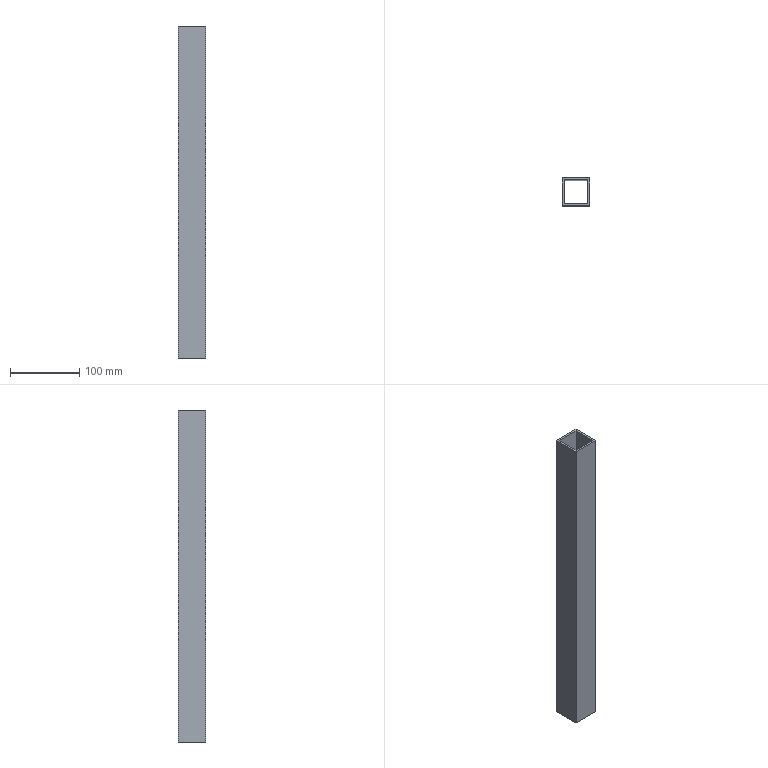Part | STEP file | BCC3 H18_2 | 1 solid | 10 faces | box 40 x 40 x 480 mm | volume 213120 mm3 | plane 10
STEP:
#1=CARTESIAN_POINT('',(0.,0.,0.));
#2=DIRECTION('',(0.,0.,1.));
#3=DIRECTION('',(1.,0.,0.));
#4=AXIS2_PLACEMENT_3D('',#1,#2,#3);
#5=CARTESIAN_POINT('',(-20.,20.,240.));
#6=VERTEX_POINT('',#5);
#7=CARTESIAN_POINT('',(-20.,-20.,240.));
#8=VERTEX_POINT('',#7);
#9=CARTESIAN_POINT('',(-20.,20.,240.));
#10=DIRECTION('',(0.,-1.,0.));
#11=VECTOR('',#10,1.);
#12=LINE('',#9,#11);
#13=CARTESIAN_POINT('',(0.,0.,240.));
#14=DIRECTION('',(0.,0.,1.));
#15=DIRECTION('',(1.,0.,0.));
#16=AXIS2_PLACEMENT_3D('',#13,#14,#15);
#17=PLANE('',#16);
#18=CARTESIAN_POINT('',(-20.,20.));
#19=DIRECTION('',(0.,-1.));
#20=VECTOR('',#19,1.);
#21=LINE('',#18,#20);
#22=(GEOMETRIC_REPRESENTATION_CONTEXT(2)PARAMETRIC_REPRESENTATION_CONTEXT()REPRESENTATION_CONTEXT('',''));
#23=DEFINITIONAL_REPRESENTATION('',(#21),#22);
#24=PCURVE('',#17,#23);
#25=CARTESIAN_POINT('',(-20.,20.,240.));
#26=DIRECTION('',(1.,0.,0.));
#27=DIRECTION('',(0.,1.,0.));
#28=AXIS2_PLACEMENT_3D('',#25,#26,#27);
#29=PLANE('',#28);
#30=CARTESIAN_POINT('',(0.,0.));
#31=DIRECTION('',(-1.,0.));
#32=VECTOR('',#31,1.);
#33=LINE('',#30,#32);
#34=(GEOMETRIC_REPRESENTATION_CONTEXT(2)PARAMETRIC_REPRESENTATION_CONTEXT()REPRESENTATION_CONTEXT('',''));
#35=DEFINITIONAL_REPRESENTATION('',(#33),#34);
#36=PCURVE('',#29,#35);
#37=SURFACE_CURVE('',#12,(#24,#36),.PCURVE_S1.);
#38=EDGE_CURVE('',#6,#8,#37,.T.);
#39=ORIENTED_EDGE('',*,*,#38,.T.);
#40=CARTESIAN_POINT('',(20.,-20.,240.));
#41=VERTEX_POINT('',#40);
#42=CARTESIAN_POINT('',(-20.,-20.,240.));
#43=DIRECTION('',(1.,0.,0.));
#44=VECTOR('',#43,1.);
#45=LINE('',#42,#44);
#46=CARTESIAN_POINT('',(-20.,-20.));
#47=DIRECTION('',(1.,0.));
#48=VECTOR('',#47,1.);
#49=LINE('',#46,#48);
#50=(GEOMETRIC_REPRESENTATION_CONTEXT(2)PARAMETRIC_REPRESENTATION_CONTEXT()REPRESENTATION_CONTEXT('',''));
#51=DEFINITIONAL_REPRESENTATION('',(#49),#50);
#52=PCURVE('',#17,#51);
#53=CARTESIAN_POINT('',(-20.,-20.,240.));
#54=DIRECTION('',(0.,1.,0.));
#55=DIRECTION('',(0.,0.,1.));
#56=AXIS2_PLACEMENT_3D('',#53,#54,#55);
#57=PLANE('',#56);
#58=CARTESIAN_POINT('',(0.,0.));
#59=DIRECTION('',(0.,1.));
#60=VECTOR('',#59,1.);
#61=LINE('',#58,#60);
#62=(GEOMETRIC_REPRESENTATION_CONTEXT(2)PARAMETRIC_REPRESENTATION_CONTEXT()REPRESENTATION_CONTEXT('',''));
#63=DEFINITIONAL_REPRESENTATION('',(#61),#62);
#64=PCURVE('',#57,#63);
#65=SURFACE_CURVE('',#45,(#52,#64),.PCURVE_S1.);
#66=EDGE_CURVE('',#8,#41,#65,.T.);
#67=ORIENTED_EDGE('',*,*,#66,.T.);
#68=CARTESIAN_POINT('',(20.,20.,240.));
#69=VERTEX_POINT('',#68);
#70=CARTESIAN_POINT('',(20.,20.,240.));
#71=DIRECTION('',(0.,1.,0.));
#72=VECTOR('',#71,1.);
#73=LINE('',#70,#72);
#74=CARTESIAN_POINT('',(20.,20.));
#75=DIRECTION('',(0.,1.));
#76=VECTOR('',#75,1.);
#77=LINE('',#74,#76);
#78=(GEOMETRIC_REPRESENTATION_CONTEXT(2)PARAMETRIC_REPRESENTATION_CONTEXT()REPRESENTATION_CONTEXT('',''));
#79=DEFINITIONAL_REPRESENTATION('',(#77),#78);
#80=PCURVE('',#17,#79);
#81=CARTESIAN_POINT('',(20.,20.,240.));
#82=DIRECTION('',(-1.,0.,0.));
#83=DIRECTION('',(0.,-1.,0.));
#84=AXIS2_PLACEMENT_3D('',#81,#82,#83);
#85=PLANE('',#84);
#86=CARTESIAN_POINT('',(0.,0.));
#87=DIRECTION('',(-1.,0.));
#88=VECTOR('',#87,1.);
#89=LINE('',#86,#88);
#90=(GEOMETRIC_REPRESENTATION_CONTEXT(2)PARAMETRIC_REPRESENTATION_CONTEXT()REPRESENTATION_CONTEXT('',''));
#91=DEFINITIONAL_REPRESENTATION('',(#89),#90);
#92=PCURVE('',#85,#91);
#93=SURFACE_CURVE('',#73,(#80,#92),.PCURVE_S1.);
#94=EDGE_CURVE('',#41,#69,#93,.T.);
#95=ORIENTED_EDGE('',*,*,#94,.T.);
#96=CARTESIAN_POINT('',(-20.,20.,240.));
#97=DIRECTION('',(-1.,0.,0.));
#98=VECTOR('',#97,1.);
#99=LINE('',#96,#98);
#100=CARTESIAN_POINT('',(-20.,20.));
#101=DIRECTION('',(-1.,0.));
#102=VECTOR('',#101,1.);
#103=LINE('',#100,#102);
#104=(GEOMETRIC_REPRESENTATION_CONTEXT(2)PARAMETRIC_REPRESENTATION_CONTEXT()REPRESENTATION_CONTEXT('',''));
#105=DEFINITIONAL_REPRESENTATION('',(#103),#104);
#106=PCURVE('',#17,#105);
#107=CARTESIAN_POINT('',(-20.,20.,240.));
#108=DIRECTION('',(0.,-1.,0.));
#109=DIRECTION('',(0.,0.,-1.));
#110=AXIS2_PLACEMENT_3D('',#107,#108,#109);
#111=PLANE('',#110);
#112=CARTESIAN_POINT('',(0.,0.));
#113=DIRECTION('',(0.,-1.));
#114=VECTOR('',#113,1.);
#115=LINE('',#112,#114);
#116=(GEOMETRIC_REPRESENTATION_CONTEXT(2)PARAMETRIC_REPRESENTATION_CONTEXT()REPRESENTATION_CONTEXT('',''));
#117=DEFINITIONAL_REPRESENTATION('',(#115),#116);
#118=PCURVE('',#111,#117);
#119=SURFACE_CURVE('',#99,(#106,#118),.PCURVE_S1.);
#120=EDGE_CURVE('',#69,#6,#119,.T.);
#121=ORIENTED_EDGE('',*,*,#120,.T.);
#122=EDGE_LOOP('',(#39,#67,#95,#121));
#123=FACE_BOUND('',#122,.T.);
#124=CARTESIAN_POINT('',(-17.,-17.,240.));
#125=VERTEX_POINT('',#124);
#126=CARTESIAN_POINT('',(17.,-17.,240.));
#127=VERTEX_POINT('',#126);
#128=CARTESIAN_POINT('',(-17.,-17.,240.));
#129=DIRECTION('',(1.,0.,0.));
#130=VECTOR('',#129,1.);
#131=LINE('',#128,#130);
#132=CARTESIAN_POINT('',(-17.,-17.));
#133=DIRECTION('',(1.,0.));
#134=VECTOR('',#133,1.);
#135=LINE('',#132,#134);
#136=(GEOMETRIC_REPRESENTATION_CONTEXT(2)PARAMETRIC_REPRESENTATION_CONTEXT()REPRESENTATION_CONTEXT('',''));
#137=DEFINITIONAL_REPRESENTATION('',(#135),#136);
#138=PCURVE('',#17,#137);
#139=CARTESIAN_POINT('',(-17.,-17.,240.));
#140=DIRECTION('',(0.,1.,0.));
#141=DIRECTION('',(-1.,0.,0.));
#142=AXIS2_PLACEMENT_3D('',#139,#140,#141);
#143=PLANE('',#142);
#144=CARTESIAN_POINT('',(0.,0.));
#145=DIRECTION('',(-1.,0.));
#146=VECTOR('',#145,1.);
#147=LINE('',#144,#146);
#148=(GEOMETRIC_REPRESENTATION_CONTEXT(2)PARAMETRIC_REPRESENTATION_CONTEXT()REPRESENTATION_CONTEXT('',''));
#149=DEFINITIONAL_REPRESENTATION('',(#147),#148);
#150=PCURVE('',#143,#149);
#151=SURFACE_CURVE('',#131,(#138,#150),.PCURVE_S1.);
#152=EDGE_CURVE('',#125,#127,#151,.T.);
#153=ORIENTED_EDGE('',*,*,#152,.F.);
#154=CARTESIAN_POINT('',(-17.,17.,240.));
#155=VERTEX_POINT('',#154);
#156=CARTESIAN_POINT('',(-17.,17.,240.));
#157=DIRECTION('',(0.,-1.,0.));
#158=VECTOR('',#157,1.);
#159=LINE('',#156,#158);
#160=CARTESIAN_POINT('',(-17.,17.));
#161=DIRECTION('',(0.,-1.));
#162=VECTOR('',#161,1.);
#163=LINE('',#160,#162);
#164=(GEOMETRIC_REPRESENTATION_CONTEXT(2)PARAMETRIC_REPRESENTATION_CONTEXT()REPRESENTATION_CONTEXT('',''));
#165=DEFINITIONAL_REPRESENTATION('',(#163),#164);
#166=PCURVE('',#17,#165);
#167=CARTESIAN_POINT('',(-17.,17.,240.));
#168=DIRECTION('',(1.,0.,0.));
#169=DIRECTION('',(0.,1.,0.));
#170=AXIS2_PLACEMENT_3D('',#167,#168,#169);
#171=PLANE('',#170);
#172=CARTESIAN_POINT('',(0.,0.));
#173=DIRECTION('',(-1.,0.));
#174=VECTOR('',#173,1.);
#175=LINE('',#172,#174);
#176=(GEOMETRIC_REPRESENTATION_CONTEXT(2)PARAMETRIC_REPRESENTATION_CONTEXT()REPRESENTATION_CONTEXT('',''));
#177=DEFINITIONAL_REPRESENTATION('',(#175),#176);
#178=PCURVE('',#171,#177);
#179=SURFACE_CURVE('',#159,(#166,#178),.PCURVE_S1.);
#180=EDGE_CURVE('',#155,#125,#179,.T.);
#181=ORIENTED_EDGE('',*,*,#180,.F.);
#182=CARTESIAN_POINT('',(17.,17.,240.));
#183=VERTEX_POINT('',#182);
#184=CARTESIAN_POINT('',(-17.,17.,240.));
#185=DIRECTION('',(-1.,0.,0.));
#186=VECTOR('',#185,1.);
#187=LINE('',#184,#186);
#188=CARTESIAN_POINT('',(-17.,17.));
#189=DIRECTION('',(-1.,0.));
#190=VECTOR('',#189,1.);
#191=LINE('',#188,#190);
#192=(GEOMETRIC_REPRESENTATION_CONTEXT(2)PARAMETRIC_REPRESENTATION_CONTEXT()REPRESENTATION_CONTEXT('',''));
#193=DEFINITIONAL_REPRESENTATION('',(#191),#192);
#194=PCURVE('',#17,#193);
#195=CARTESIAN_POINT('',(-17.,17.,240.));
#196=DIRECTION('',(0.,-1.,0.));
#197=DIRECTION('',(0.,0.,-1.));
#198=AXIS2_PLACEMENT_3D('',#195,#196,#197);
#199=PLANE('',#198);
#200=CARTESIAN_POINT('',(0.,0.));
#201=DIRECTION('',(0.,-1.));
#202=VECTOR('',#201,1.);
#203=LINE('',#200,#202);
#204=(GEOMETRIC_REPRESENTATION_CONTEXT(2)PARAMETRIC_REPRESENTATION_CONTEXT()REPRESENTATION_CONTEXT('',''));
#205=DEFINITIONAL_REPRESENTATION('',(#203),#204);
#206=PCURVE('',#199,#205);
#207=SURFACE_CURVE('',#187,(#194,#206),.PCURVE_S1.);
#208=EDGE_CURVE('',#183,#155,#207,.T.);
#209=ORIENTED_EDGE('',*,*,#208,.F.);
#210=CARTESIAN_POINT('',(17.,17.,240.));
#211=DIRECTION('',(0.,1.,0.));
#212=VECTOR('',#211,1.);
#213=LINE('',#210,#212);
#214=CARTESIAN_POINT('',(17.,17.));
#215=DIRECTION('',(0.,1.));
#216=VECTOR('',#215,1.);
#217=LINE('',#214,#216);
#218=(GEOMETRIC_REPRESENTATION_CONTEXT(2)PARAMETRIC_REPRESENTATION_CONTEXT()REPRESENTATION_CONTEXT('',''));
#219=DEFINITIONAL_REPRESENTATION('',(#217),#218);
#220=PCURVE('',#17,#219);
#221=CARTESIAN_POINT('',(17.,17.,240.));
#222=DIRECTION('',(-1.,0.,0.));
#223=DIRECTION('',(0.,-1.,0.));
#224=AXIS2_PLACEMENT_3D('',#221,#222,#223);
#225=PLANE('',#224);
#226=CARTESIAN_POINT('',(0.,0.));
#227=DIRECTION('',(-1.,0.));
#228=VECTOR('',#227,1.);
#229=LINE('',#226,#228);
#230=(GEOMETRIC_REPRESENTATION_CONTEXT(2)PARAMETRIC_REPRESENTATION_CONTEXT()REPRESENTATION_CONTEXT('',''));
#231=DEFINITIONAL_REPRESENTATION('',(#229),#230);
#232=PCURVE('',#225,#231);
#233=SURFACE_CURVE('',#213,(#220,#232),.PCURVE_S1.);
#234=EDGE_CURVE('',#127,#183,#233,.T.);
#235=ORIENTED_EDGE('',*,*,#234,.F.);
#236=EDGE_LOOP('',(#153,#181,#209,#235));
#237=FACE_BOUND('',#236,.T.);
#238=ADVANCED_FACE('',(#123,#237),#17,.T.);
#239=CARTESIAN_POINT('',(-20.,20.,-240.));
#240=VERTEX_POINT('',#239);
#241=CARTESIAN_POINT('',(-20.,-20.,-240.));
#242=VERTEX_POINT('',#241);
#243=CARTESIAN_POINT('',(-20.,20.,-240.));
#244=DIRECTION('',(0.,-1.,0.));
#245=VECTOR('',#244,1.);
#246=LINE('',#243,#245);
#247=CARTESIAN_POINT('',(0.,0.,-240.));
#248=DIRECTION('',(0.,0.,1.));
#249=DIRECTION('',(1.,0.,0.));
#250=AXIS2_PLACEMENT_3D('',#247,#248,#249);
#251=PLANE('',#250);
#252=CARTESIAN_POINT('',(-20.,20.));
#253=DIRECTION('',(0.,-1.));
#254=VECTOR('',#253,1.);
#255=LINE('',#252,#254);
#256=(GEOMETRIC_REPRESENTATION_CONTEXT(2)PARAMETRIC_REPRESENTATION_CONTEXT()REPRESENTATION_CONTEXT('',''));
#257=DEFINITIONAL_REPRESENTATION('',(#255),#256);
#258=PCURVE('',#251,#257);
#259=CARTESIAN_POINT('',(0.,-480.));
#260=DIRECTION('',(-1.,0.));
#261=VECTOR('',#260,1.);
#262=LINE('',#259,#261);
#263=(GEOMETRIC_REPRESENTATION_CONTEXT(2)PARAMETRIC_REPRESENTATION_CONTEXT()REPRESENTATION_CONTEXT('',''));
#264=DEFINITIONAL_REPRESENTATION('',(#262),#263);
#265=PCURVE('',#29,#264);
#266=SURFACE_CURVE('',#246,(#258,#265),.PCURVE_S1.);
#267=EDGE_CURVE('',#240,#242,#266,.T.);
#268=ORIENTED_EDGE('',*,*,#267,.F.);
#269=CARTESIAN_POINT('',(20.,20.,-240.));
#270=VERTEX_POINT('',#269);
#271=CARTESIAN_POINT('',(-20.,20.,-240.));
#272=DIRECTION('',(-1.,0.,0.));
#273=VECTOR('',#272,1.);
#274=LINE('',#271,#273);
#275=CARTESIAN_POINT('',(-20.,20.));
#276=DIRECTION('',(-1.,0.));
#277=VECTOR('',#276,1.);
#278=LINE('',#275,#277);
#279=(GEOMETRIC_REPRESENTATION_CONTEXT(2)PARAMETRIC_REPRESENTATION_CONTEXT()REPRESENTATION_CONTEXT('',''));
#280=DEFINITIONAL_REPRESENTATION('',(#278),#279);
#281=PCURVE('',#251,#280);
#282=CARTESIAN_POINT('',(480.,0.));
#283=DIRECTION('',(0.,-1.));
#284=VECTOR('',#283,1.);
#285=LINE('',#282,#284);
#286=(GEOMETRIC_REPRESENTATION_CONTEXT(2)PARAMETRIC_REPRESENTATION_CONTEXT()REPRESENTATION_CONTEXT('',''));
#287=DEFINITIONAL_REPRESENTATION('',(#285),#286);
#288=PCURVE('',#111,#287);
#289=SURFACE_CURVE('',#274,(#281,#288),.PCURVE_S1.);
#290=EDGE_CURVE('',#270,#240,#289,.T.);
#291=ORIENTED_EDGE('',*,*,#290,.F.);
#292=CARTESIAN_POINT('',(20.,-20.,-240.));
#293=VERTEX_POINT('',#292);
#294=CARTESIAN_POINT('',(20.,20.,-240.));
#295=DIRECTION('',(0.,1.,0.));
#296=VECTOR('',#295,1.);
#297=LINE('',#294,#296);
#298=CARTESIAN_POINT('',(20.,20.));
#299=DIRECTION('',(0.,1.));
#300=VECTOR('',#299,1.);
#301=LINE('',#298,#300);
#302=(GEOMETRIC_REPRESENTATION_CONTEXT(2)PARAMETRIC_REPRESENTATION_CONTEXT()REPRESENTATION_CONTEXT('',''));
#303=DEFINITIONAL_REPRESENTATION('',(#301),#302);
#304=PCURVE('',#251,#303);
#305=CARTESIAN_POINT('',(0.,-480.));
#306=DIRECTION('',(-1.,0.));
#307=VECTOR('',#306,1.);
#308=LINE('',#305,#307);
#309=(GEOMETRIC_REPRESENTATION_CONTEXT(2)PARAMETRIC_REPRESENTATION_CONTEXT()REPRESENTATION_CONTEXT('',''));
#310=DEFINITIONAL_REPRESENTATION('',(#308),#309);
#311=PCURVE('',#85,#310);
#312=SURFACE_CURVE('',#297,(#304,#311),.PCURVE_S1.);
#313=EDGE_CURVE('',#293,#270,#312,.T.);
#314=ORIENTED_EDGE('',*,*,#313,.F.);
#315=CARTESIAN_POINT('',(-20.,-20.,-240.));
#316=DIRECTION('',(1.,0.,0.));
#317=VECTOR('',#316,1.);
#318=LINE('',#315,#317);
#319=CARTESIAN_POINT('',(-20.,-20.));
#320=DIRECTION('',(1.,0.));
#321=VECTOR('',#320,1.);
#322=LINE('',#319,#321);
#323=(GEOMETRIC_REPRESENTATION_CONTEXT(2)PARAMETRIC_REPRESENTATION_CONTEXT()REPRESENTATION_CONTEXT('',''));
#324=DEFINITIONAL_REPRESENTATION('',(#322),#323);
#325=PCURVE('',#251,#324);
#326=CARTESIAN_POINT('',(-480.,0.));
#327=DIRECTION('',(0.,1.));
#328=VECTOR('',#327,1.);
#329=LINE('',#326,#328);
#330=(GEOMETRIC_REPRESENTATION_CONTEXT(2)PARAMETRIC_REPRESENTATION_CONTEXT()REPRESENTATION_CONTEXT('',''));
#331=DEFINITIONAL_REPRESENTATION('',(#329),#330);
#332=PCURVE('',#57,#331);
#333=SURFACE_CURVE('',#318,(#325,#332),.PCURVE_S1.);
#334=EDGE_CURVE('',#242,#293,#333,.T.);
#335=ORIENTED_EDGE('',*,*,#334,.F.);
#336=EDGE_LOOP('',(#268,#291,#314,#335));
#337=FACE_BOUND('',#336,.T.);
#338=CARTESIAN_POINT('',(-17.,17.,-240.));
#339=VERTEX_POINT('',#338);
#340=CARTESIAN_POINT('',(-17.,-17.,-240.));
#341=VERTEX_POINT('',#340);
#342=CARTESIAN_POINT('',(-17.,17.,-240.));
#343=DIRECTION('',(0.,-1.,0.));
#344=VECTOR('',#343,1.);
#345=LINE('',#342,#344);
#346=CARTESIAN_POINT('',(-17.,17.));
#347=DIRECTION('',(0.,-1.));
#348=VECTOR('',#347,1.);
#349=LINE('',#346,#348);
#350=(GEOMETRIC_REPRESENTATION_CONTEXT(2)PARAMETRIC_REPRESENTATION_CONTEXT()REPRESENTATION_CONTEXT('',''));
#351=DEFINITIONAL_REPRESENTATION('',(#349),#350);
#352=PCURVE('',#251,#351);
#353=CARTESIAN_POINT('',(0.,-480.));
#354=DIRECTION('',(-1.,0.));
#355=VECTOR('',#354,1.);
#356=LINE('',#353,#355);
#357=(GEOMETRIC_REPRESENTATION_CONTEXT(2)PARAMETRIC_REPRESENTATION_CONTEXT()REPRESENTATION_CONTEXT('',''));
#358=DEFINITIONAL_REPRESENTATION('',(#356),#357);
#359=PCURVE('',#171,#358);
#360=SURFACE_CURVE('',#345,(#352,#359),.PCURVE_S1.);
#361=EDGE_CURVE('',#339,#341,#360,.T.);
#362=ORIENTED_EDGE('',*,*,#361,.T.);
#363=CARTESIAN_POINT('',(17.,-17.,-240.));
#364=VERTEX_POINT('',#363);
#365=CARTESIAN_POINT('',(-17.,-17.,-240.));
#366=DIRECTION('',(1.,0.,0.));
#367=VECTOR('',#366,1.);
#368=LINE('',#365,#367);
#369=CARTESIAN_POINT('',(-17.,-17.));
#370=DIRECTION('',(1.,0.));
#371=VECTOR('',#370,1.);
#372=LINE('',#369,#371);
#373=(GEOMETRIC_REPRESENTATION_CONTEXT(2)PARAMETRIC_REPRESENTATION_CONTEXT()REPRESENTATION_CONTEXT('',''));
#374=DEFINITIONAL_REPRESENTATION('',(#372),#373);
#375=PCURVE('',#251,#374);
#376=CARTESIAN_POINT('',(0.,-480.));
#377=DIRECTION('',(-1.,0.));
#378=VECTOR('',#377,1.);
#379=LINE('',#376,#378);
#380=(GEOMETRIC_REPRESENTATION_CONTEXT(2)PARAMETRIC_REPRESENTATION_CONTEXT()REPRESENTATION_CONTEXT('',''));
#381=DEFINITIONAL_REPRESENTATION('',(#379),#380);
#382=PCURVE('',#143,#381);
#383=SURFACE_CURVE('',#368,(#375,#382),.PCURVE_S1.);
#384=EDGE_CURVE('',#341,#364,#383,.T.);
#385=ORIENTED_EDGE('',*,*,#384,.T.);
#386=CARTESIAN_POINT('',(17.,17.,-240.));
#387=VERTEX_POINT('',#386);
#388=CARTESIAN_POINT('',(17.,17.,-240.));
#389=DIRECTION('',(0.,1.,0.));
#390=VECTOR('',#389,1.);
#391=LINE('',#388,#390);
#392=CARTESIAN_POINT('',(17.,17.));
#393=DIRECTION('',(0.,1.));
#394=VECTOR('',#393,1.);
#395=LINE('',#392,#394);
#396=(GEOMETRIC_REPRESENTATION_CONTEXT(2)PARAMETRIC_REPRESENTATION_CONTEXT()REPRESENTATION_CONTEXT('',''));
#397=DEFINITIONAL_REPRESENTATION('',(#395),#396);
#398=PCURVE('',#251,#397);
#399=CARTESIAN_POINT('',(0.,-480.));
#400=DIRECTION('',(-1.,0.));
#401=VECTOR('',#400,1.);
#402=LINE('',#399,#401);
#403=(GEOMETRIC_REPRESENTATION_CONTEXT(2)PARAMETRIC_REPRESENTATION_CONTEXT()REPRESENTATION_CONTEXT('',''));
#404=DEFINITIONAL_REPRESENTATION('',(#402),#403);
#405=PCURVE('',#225,#404);
#406=SURFACE_CURVE('',#391,(#398,#405),.PCURVE_S1.);
#407=EDGE_CURVE('',#364,#387,#406,.T.);
#408=ORIENTED_EDGE('',*,*,#407,.T.);
#409=CARTESIAN_POINT('',(-17.,17.,-240.));
#410=DIRECTION('',(-1.,0.,0.));
#411=VECTOR('',#410,1.);
#412=LINE('',#409,#411);
#413=CARTESIAN_POINT('',(-17.,17.));
#414=DIRECTION('',(-1.,0.));
#415=VECTOR('',#414,1.);
#416=LINE('',#413,#415);
#417=(GEOMETRIC_REPRESENTATION_CONTEXT(2)PARAMETRIC_REPRESENTATION_CONTEXT()REPRESENTATION_CONTEXT('',''));
#418=DEFINITIONAL_REPRESENTATION('',(#416),#417);
#419=PCURVE('',#251,#418);
#420=CARTESIAN_POINT('',(480.,0.));
#421=DIRECTION('',(0.,-1.));
#422=VECTOR('',#421,1.);
#423=LINE('',#420,#422);
#424=(GEOMETRIC_REPRESENTATION_CONTEXT(2)PARAMETRIC_REPRESENTATION_CONTEXT()REPRESENTATION_CONTEXT('',''));
#425=DEFINITIONAL_REPRESENTATION('',(#423),#424);
#426=PCURVE('',#199,#425);
#427=SURFACE_CURVE('',#412,(#419,#426),.PCURVE_S1.);
#428=EDGE_CURVE('',#387,#339,#427,.T.);
#429=ORIENTED_EDGE('',*,*,#428,.T.);
#430=EDGE_LOOP('',(#362,#385,#408,#429));
#431=FACE_BOUND('',#430,.T.);
#432=ADVANCED_FACE('',(#337,#431),#251,.F.);
#433=ORIENTED_EDGE('',*,*,#267,.T.);
#434=CARTESIAN_POINT('',(-20.,-20.,240.));
#435=DIRECTION('',(0.,0.,-1.));
#436=VECTOR('',#435,1.);
#437=LINE('',#434,#436);
#438=CARTESIAN_POINT('',(-40.,0.));
#439=DIRECTION('',(0.,-1.));
#440=VECTOR('',#439,1.);
#441=LINE('',#438,#440);
#442=(GEOMETRIC_REPRESENTATION_CONTEXT(2)PARAMETRIC_REPRESENTATION_CONTEXT()REPRESENTATION_CONTEXT('',''));
#443=DEFINITIONAL_REPRESENTATION('',(#441),#442);
#444=PCURVE('',#29,#443);
#445=CARTESIAN_POINT('',(0.,0.));
#446=DIRECTION('',(-1.,0.));
#447=VECTOR('',#446,1.);
#448=LINE('',#445,#447);
#449=(GEOMETRIC_REPRESENTATION_CONTEXT(2)PARAMETRIC_REPRESENTATION_CONTEXT()REPRESENTATION_CONTEXT('',''));
#450=DEFINITIONAL_REPRESENTATION('',(#448),#449);
#451=PCURVE('',#57,#450);
#452=SURFACE_CURVE('',#437,(#444,#451),.PCURVE_S1.);
#453=EDGE_CURVE('',#8,#242,#452,.T.);
#454=ORIENTED_EDGE('',*,*,#453,.F.);
#455=ORIENTED_EDGE('',*,*,#38,.F.);
#456=CARTESIAN_POINT('',(-20.,20.,240.));
#457=DIRECTION('',(0.,0.,-1.));
#458=VECTOR('',#457,1.);
#459=LINE('',#456,#458);
#460=CARTESIAN_POINT('',(0.,0.));
#461=DIRECTION('',(0.,-1.));
#462=VECTOR('',#461,1.);
#463=LINE('',#460,#462);
#464=(GEOMETRIC_REPRESENTATION_CONTEXT(2)PARAMETRIC_REPRESENTATION_CONTEXT()REPRESENTATION_CONTEXT('',''));
#465=DEFINITIONAL_REPRESENTATION('',(#463),#464);
#466=PCURVE('',#29,#465);
#467=CARTESIAN_POINT('',(0.,0.));
#468=DIRECTION('',(1.,0.));
#469=VECTOR('',#468,1.);
#470=LINE('',#467,#469);
#471=(GEOMETRIC_REPRESENTATION_CONTEXT(2)PARAMETRIC_REPRESENTATION_CONTEXT()REPRESENTATION_CONTEXT('',''));
#472=DEFINITIONAL_REPRESENTATION('',(#470),#471);
#473=PCURVE('',#111,#472);
#474=SURFACE_CURVE('',#459,(#466,#473),.PCURVE_S1.);
#475=EDGE_CURVE('',#6,#240,#474,.T.);
#476=ORIENTED_EDGE('',*,*,#475,.T.);
#477=EDGE_LOOP('',(#433,#454,#455,#476));
#478=FACE_BOUND('',#477,.T.);
#479=ADVANCED_FACE('',(#478),#29,.F.);
#480=ORIENTED_EDGE('',*,*,#334,.T.);
#481=CARTESIAN_POINT('',(20.,-20.,240.));
#482=DIRECTION('',(0.,0.,-1.));
#483=VECTOR('',#482,1.);
#484=LINE('',#481,#483);
#485=CARTESIAN_POINT('',(0.,40.));
#486=DIRECTION('',(-1.,0.));
#487=VECTOR('',#486,1.);
#488=LINE('',#485,#487);
#489=(GEOMETRIC_REPRESENTATION_CONTEXT(2)PARAMETRIC_REPRESENTATION_CONTEXT()REPRESENTATION_CONTEXT('',''));
#490=DEFINITIONAL_REPRESENTATION('',(#488),#489);
#491=PCURVE('',#57,#490);
#492=CARTESIAN_POINT('',(40.,0.));
#493=DIRECTION('',(0.,-1.));
#494=VECTOR('',#493,1.);
#495=LINE('',#492,#494);
#496=(GEOMETRIC_REPRESENTATION_CONTEXT(2)PARAMETRIC_REPRESENTATION_CONTEXT()REPRESENTATION_CONTEXT('',''));
#497=DEFINITIONAL_REPRESENTATION('',(#495),#496);
#498=PCURVE('',#85,#497);
#499=SURFACE_CURVE('',#484,(#491,#498),.PCURVE_S1.);
#500=EDGE_CURVE('',#41,#293,#499,.T.);
#501=ORIENTED_EDGE('',*,*,#500,.F.);
#502=ORIENTED_EDGE('',*,*,#66,.F.);
#503=ORIENTED_EDGE('',*,*,#453,.T.);
#504=EDGE_LOOP('',(#480,#501,#502,#503));
#505=FACE_BOUND('',#504,.T.);
#506=ADVANCED_FACE('',(#505),#57,.F.);
#507=ORIENTED_EDGE('',*,*,#313,.T.);
#508=CARTESIAN_POINT('',(20.,20.,240.));
#509=DIRECTION('',(0.,0.,-1.));
#510=VECTOR('',#509,1.);
#511=LINE('',#508,#510);
#512=CARTESIAN_POINT('',(0.,0.));
#513=DIRECTION('',(0.,-1.));
#514=VECTOR('',#513,1.);
#515=LINE('',#512,#514);
#516=(GEOMETRIC_REPRESENTATION_CONTEXT(2)PARAMETRIC_REPRESENTATION_CONTEXT()REPRESENTATION_CONTEXT('',''));
#517=DEFINITIONAL_REPRESENTATION('',(#515),#516);
#518=PCURVE('',#85,#517);
#519=CARTESIAN_POINT('',(0.,40.));
#520=DIRECTION('',(1.,0.));
#521=VECTOR('',#520,1.);
#522=LINE('',#519,#521);
#523=(GEOMETRIC_REPRESENTATION_CONTEXT(2)PARAMETRIC_REPRESENTATION_CONTEXT()REPRESENTATION_CONTEXT('',''));
#524=DEFINITIONAL_REPRESENTATION('',(#522),#523);
#525=PCURVE('',#111,#524);
#526=SURFACE_CURVE('',#511,(#518,#525),.PCURVE_S1.);
#527=EDGE_CURVE('',#69,#270,#526,.T.);
#528=ORIENTED_EDGE('',*,*,#527,.F.);
#529=ORIENTED_EDGE('',*,*,#94,.F.);
#530=ORIENTED_EDGE('',*,*,#500,.T.);
#531=EDGE_LOOP('',(#507,#528,#529,#530));
#532=FACE_BOUND('',#531,.T.);
#533=ADVANCED_FACE('',(#532),#85,.F.);
#534=ORIENTED_EDGE('',*,*,#290,.T.);
#535=ORIENTED_EDGE('',*,*,#475,.F.);
#536=ORIENTED_EDGE('',*,*,#120,.F.);
#537=ORIENTED_EDGE('',*,*,#527,.T.);
#538=EDGE_LOOP('',(#534,#535,#536,#537));
#539=FACE_BOUND('',#538,.T.);
#540=ADVANCED_FACE('',(#539),#111,.F.);
#541=ORIENTED_EDGE('',*,*,#361,.F.);
#542=CARTESIAN_POINT('',(-17.,17.,240.));
#543=DIRECTION('',(0.,0.,-1.));
#544=VECTOR('',#543,1.);
#545=LINE('',#542,#544);
#546=CARTESIAN_POINT('',(0.,0.));
#547=DIRECTION('',(0.,-1.));
#548=VECTOR('',#547,1.);
#549=LINE('',#546,#548);
#550=(GEOMETRIC_REPRESENTATION_CONTEXT(2)PARAMETRIC_REPRESENTATION_CONTEXT()REPRESENTATION_CONTEXT('',''));
#551=DEFINITIONAL_REPRESENTATION('',(#549),#550);
#552=PCURVE('',#171,#551);
#553=CARTESIAN_POINT('',(0.,0.));
#554=DIRECTION('',(1.,0.));
#555=VECTOR('',#554,1.);
#556=LINE('',#553,#555);
#557=(GEOMETRIC_REPRESENTATION_CONTEXT(2)PARAMETRIC_REPRESENTATION_CONTEXT()REPRESENTATION_CONTEXT('',''));
#558=DEFINITIONAL_REPRESENTATION('',(#556),#557);
#559=PCURVE('',#199,#558);
#560=SURFACE_CURVE('',#545,(#552,#559),.PCURVE_S1.);
#561=EDGE_CURVE('',#155,#339,#560,.T.);
#562=ORIENTED_EDGE('',*,*,#561,.F.);
#563=ORIENTED_EDGE('',*,*,#180,.T.);
#564=CARTESIAN_POINT('',(-17.,-17.,240.));
#565=DIRECTION('',(0.,0.,-1.));
#566=VECTOR('',#565,1.);
#567=LINE('',#564,#566);
#568=CARTESIAN_POINT('',(-34.,0.));
#569=DIRECTION('',(0.,-1.));
#570=VECTOR('',#569,1.);
#571=LINE('',#568,#570);
#572=(GEOMETRIC_REPRESENTATION_CONTEXT(2)PARAMETRIC_REPRESENTATION_CONTEXT()REPRESENTATION_CONTEXT('',''));
#573=DEFINITIONAL_REPRESENTATION('',(#571),#572);
#574=PCURVE('',#171,#573);
#575=CARTESIAN_POINT('',(0.,0.));
#576=DIRECTION('',(0.,-1.));
#577=VECTOR('',#576,1.);
#578=LINE('',#575,#577);
#579=(GEOMETRIC_REPRESENTATION_CONTEXT(2)PARAMETRIC_REPRESENTATION_CONTEXT()REPRESENTATION_CONTEXT('',''));
#580=DEFINITIONAL_REPRESENTATION('',(#578),#579);
#581=PCURVE('',#143,#580);
#582=SURFACE_CURVE('',#567,(#574,#581),.PCURVE_S1.);
#583=EDGE_CURVE('',#125,#341,#582,.T.);
#584=ORIENTED_EDGE('',*,*,#583,.T.);
#585=EDGE_LOOP('',(#541,#562,#563,#584));
#586=FACE_BOUND('',#585,.T.);
#587=ADVANCED_FACE('',(#586),#171,.T.);
#588=ORIENTED_EDGE('',*,*,#384,.F.);
#589=ORIENTED_EDGE('',*,*,#583,.F.);
#590=ORIENTED_EDGE('',*,*,#152,.T.);
#591=CARTESIAN_POINT('',(17.,-17.,240.));
#592=DIRECTION('',(0.,0.,-1.));
#593=VECTOR('',#592,1.);
#594=LINE('',#591,#593);
#595=CARTESIAN_POINT('',(-34.,0.));
#596=DIRECTION('',(0.,-1.));
#597=VECTOR('',#596,1.);
#598=LINE('',#595,#597);
#599=(GEOMETRIC_REPRESENTATION_CONTEXT(2)PARAMETRIC_REPRESENTATION_CONTEXT()REPRESENTATION_CONTEXT('',''));
#600=DEFINITIONAL_REPRESENTATION('',(#598),#599);
#601=PCURVE('',#143,#600);
#602=CARTESIAN_POINT('',(34.,0.));
#603=DIRECTION('',(0.,-1.));
#604=VECTOR('',#603,1.);
#605=LINE('',#602,#604);
#606=(GEOMETRIC_REPRESENTATION_CONTEXT(2)PARAMETRIC_REPRESENTATION_CONTEXT()REPRESENTATION_CONTEXT('',''));
#607=DEFINITIONAL_REPRESENTATION('',(#605),#606);
#608=PCURVE('',#225,#607);
#609=SURFACE_CURVE('',#594,(#601,#608),.PCURVE_S1.);
#610=EDGE_CURVE('',#127,#364,#609,.T.);
#611=ORIENTED_EDGE('',*,*,#610,.T.);
#612=EDGE_LOOP('',(#588,#589,#590,#611));
#613=FACE_BOUND('',#612,.T.);
#614=ADVANCED_FACE('',(#613),#143,.T.);
#615=ORIENTED_EDGE('',*,*,#407,.F.);
#616=ORIENTED_EDGE('',*,*,#610,.F.);
#617=ORIENTED_EDGE('',*,*,#234,.T.);
#618=CARTESIAN_POINT('',(17.,17.,240.));
#619=DIRECTION('',(0.,0.,-1.));
#620=VECTOR('',#619,1.);
#621=LINE('',#618,#620);
#622=CARTESIAN_POINT('',(0.,0.));
#623=DIRECTION('',(0.,-1.));
#624=VECTOR('',#623,1.);
#625=LINE('',#622,#624);
#626=(GEOMETRIC_REPRESENTATION_CONTEXT(2)PARAMETRIC_REPRESENTATION_CONTEXT()REPRESENTATION_CONTEXT('',''));
#627=DEFINITIONAL_REPRESENTATION('',(#625),#626);
#628=PCURVE('',#225,#627);
#629=CARTESIAN_POINT('',(0.,34.));
#630=DIRECTION('',(1.,0.));
#631=VECTOR('',#630,1.);
#632=LINE('',#629,#631);
#633=(GEOMETRIC_REPRESENTATION_CONTEXT(2)PARAMETRIC_REPRESENTATION_CONTEXT()REPRESENTATION_CONTEXT('',''));
#634=DEFINITIONAL_REPRESENTATION('',(#632),#633);
#635=PCURVE('',#199,#634);
#636=SURFACE_CURVE('',#621,(#628,#635),.PCURVE_S1.);
#637=EDGE_CURVE('',#183,#387,#636,.T.);
#638=ORIENTED_EDGE('',*,*,#637,.T.);
#639=EDGE_LOOP('',(#615,#616,#617,#638));
#640=FACE_BOUND('',#639,.T.);
#641=ADVANCED_FACE('',(#640),#225,.T.);
#642=ORIENTED_EDGE('',*,*,#428,.F.);
#643=ORIENTED_EDGE('',*,*,#637,.F.);
#644=ORIENTED_EDGE('',*,*,#208,.T.);
#645=ORIENTED_EDGE('',*,*,#561,.T.);
#646=EDGE_LOOP('',(#642,#643,#644,#645));
#647=FACE_BOUND('',#646,.T.);
#648=ADVANCED_FACE('',(#647),#199,.T.);
#649=CLOSED_SHELL('',(#238,#432,#479,#506,#533,#540,#587,#614,#641,#648));
#650=MANIFOLD_SOLID_BREP('',#649);
#651=(LENGTH_UNIT()NAMED_UNIT(*)SI_UNIT(.MILLI.,.METRE.));
#652=UNCERTAINTY_MEASURE_WITH_UNIT(LENGTH_MEASURE(0.0000001),#651,'','');
#653=(NAMED_UNIT(*)PLANE_ANGLE_UNIT()SI_UNIT($,.RADIAN.));
#654=(NAMED_UNIT(*)SI_UNIT($,.STERADIAN.)SOLID_ANGLE_UNIT());
#655=(GEOMETRIC_REPRESENTATION_CONTEXT(3)GLOBAL_UNCERTAINTY_ASSIGNED_CONTEXT((#652))GLOBAL_UNIT_ASSIGNED_CONTEXT((#651,#653,#654))REPRESENTATION_CONTEXT('',''));
#656=ADVANCED_BREP_SHAPE_REPRESENTATION('',(#4,#650),#655);